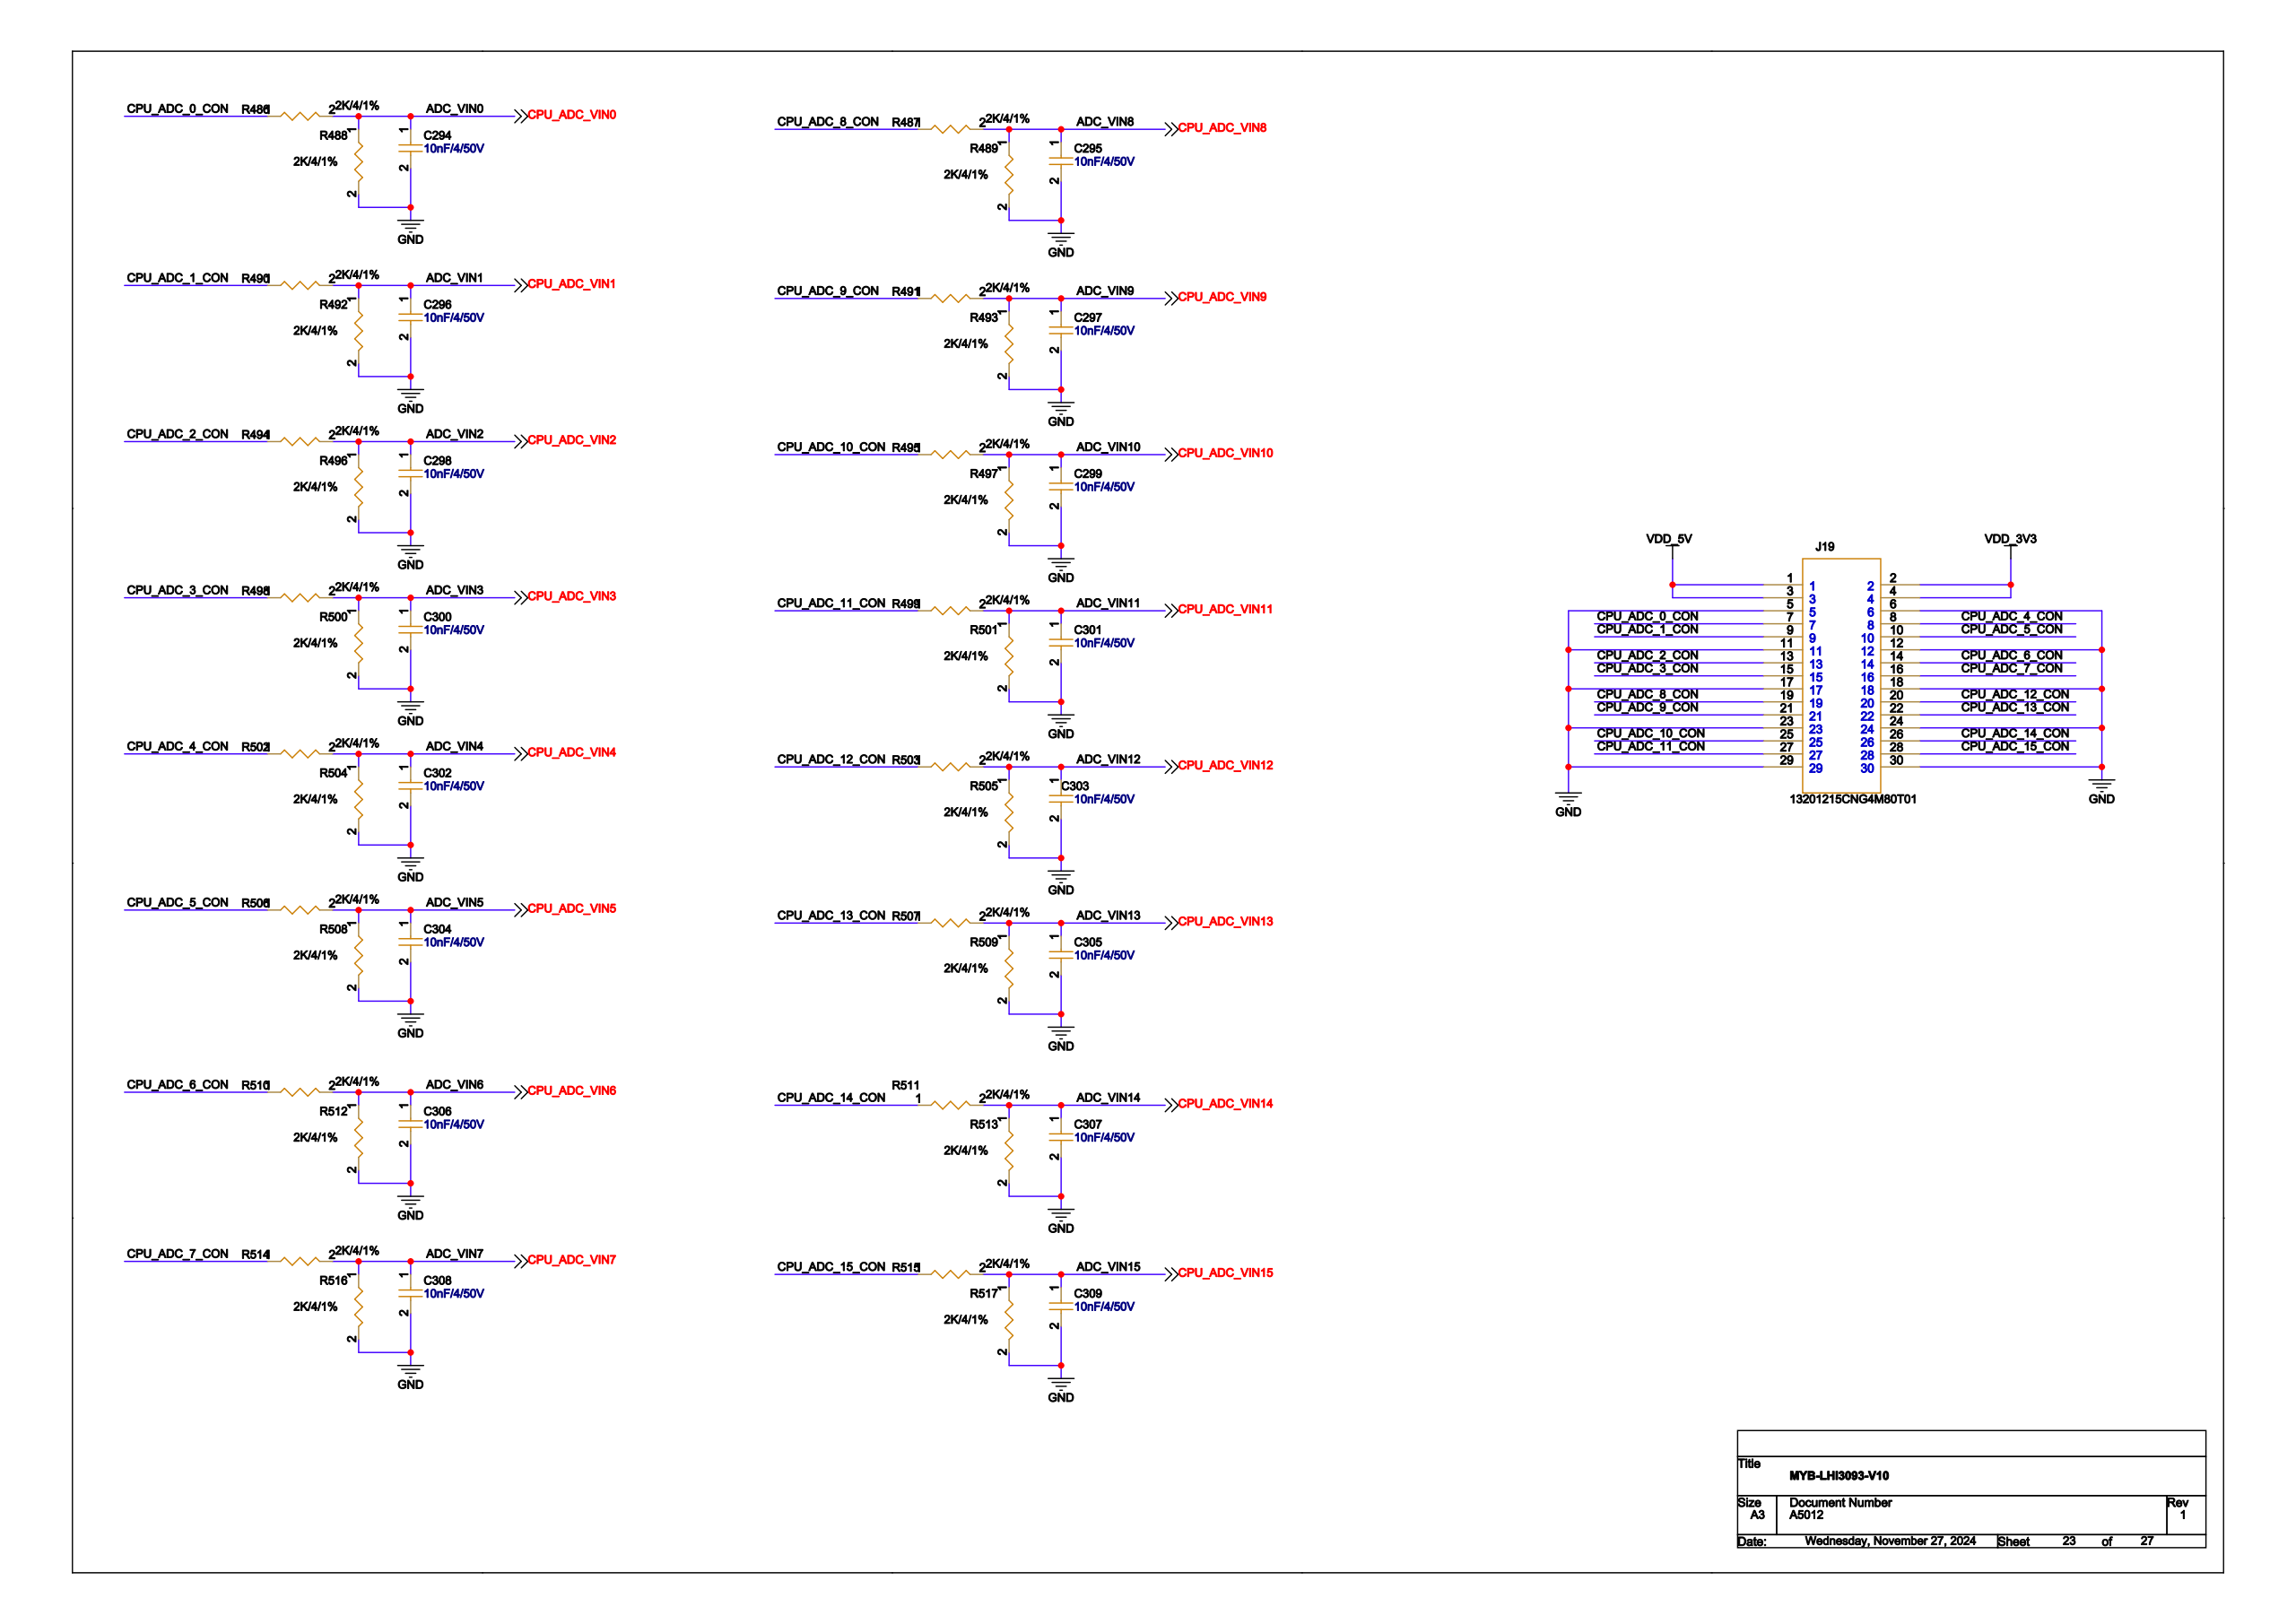Circuit board | Cadence Allegro | 1159 parts | 708 nets | one sheet of the schematic
Parts on this sheet (reference | value | footprint):
C294 | 10nF/4/50V | C0402
C295 | 10nF/4/50V | C0402
C296 | 10nF/4/50V | C0402
C297 | 10nF/4/50V | C0402
C298 | 10nF/4/50V | C0402
C299 | 10nF/4/50V | C0402
C300 | 10nF/4/50V | C0402
C301 | 10nF/4/50V | C0402
C302 | 10nF/4/50V | C0402
C303 | 10nF/4/50V | C0402
C304 | 10nF/4/50V | C0402
C305 | 10nF/4/50V | C0402
C306 | 10nF/4/50V | C0402
C307 | 10nF/4/50V | C0402
C308 | 10nF/4/50V | C0402
C309 | 10nF/4/50V | C0402
J19 | 13201215CNG4M80T01 | CONN2X15-2_00-SMD
R488 | 2K/4/1% | R0402
R489 | 2K/4/1% | R0402
R492 | 2K/4/1% | R0402
R493 | 2K/4/1% | R0402
R496 | 2K/4/1% | R0402
R497 | 2K/4/1% | R0402
R500 | 2K/4/1% | R0402
R501 | 2K/4/1% | R0402
R504 | 2K/4/1% | R0402
R505 | 2K/4/1% | R0402
R508 | 2K/4/1% | R0402
R509 | 2K/4/1% | R0402
R512 | 2K/4/1% | R0402
R513 | 2K/4/1% | R0402
R516 | 2K/4/1% | R0402
R517 | 2K/4/1% | R0402
Nets of these parts (net: part-pin ...):
GND: C294-2 C295-2 C296-2 C297-2 C298-2 C299-2 C300-2 C301-2 C302-2 C303-2 C304-2 C305-2 C306-2 C307-2 C308-2 C309-2 R488-2 R489-2 R492-2 R493-2 R496-2 R497-2 R500-2 R501-2 R504-2 R505-2 R508-2 R509-2 R512-2 R513-2 R516-2 R517-2 J19-5 J19-6 J19-11 J19-12 J19-17 J19-18 J19-23 J19-24 J19-29 J19-30
VDD_5V: J19-1 J19-3
VDD_3V3: J19-2 J19-4
CPU_ADC_VIN0: C294-1 R488-1
CPU_ADC_VIN8: C295-1 R489-1
CPU_ADC_VIN1: C296-1 R492-1
CPU_ADC_VIN9: C297-1 R493-1
CPU_ADC_VIN2: C298-1 R496-1
CPU_ADC_VIN10: C299-1 R497-1
CPU_ADC_VIN3: C300-1 R500-1
CPU_ADC_VIN11: C301-1 R501-1
CPU_ADC_VIN4: C302-1 R504-1
CPU_ADC_VIN12: C303-1 R505-1
CPU_ADC_VIN5: C304-1 R508-1
CPU_ADC_VIN13: C305-1 R509-1
CPU_ADC_VIN6: C306-1 R512-1
CPU_ADC_VIN14: C307-1 R513-1
CPU_ADC_VIN7: C308-1 R516-1
CPU_ADC_VIN15: C309-1 R517-1
CPU_ADC_5_CON: J19-10
CPU_ADC_2_CON: J19-13
CPU_ADC_6_CON: J19-14
CPU_ADC_3_CON: J19-15
CPU_ADC_7_CON: J19-16
CPU_ADC_8_CON: J19-19
CPU_ADC_12_CON: J19-20
CPU_ADC_9_CON: J19-21
CPU_ADC_13_CON: J19-22
CPU_ADC_10_CON: J19-25
CPU_ADC_14_CON: J19-26
CPU_ADC_11_CON: J19-27
CPU_ADC_15_CON: J19-28
CPU_ADC_0_CON: J19-7
CPU_ADC_4_CON: J19-8
CPU_ADC_1_CON: J19-9